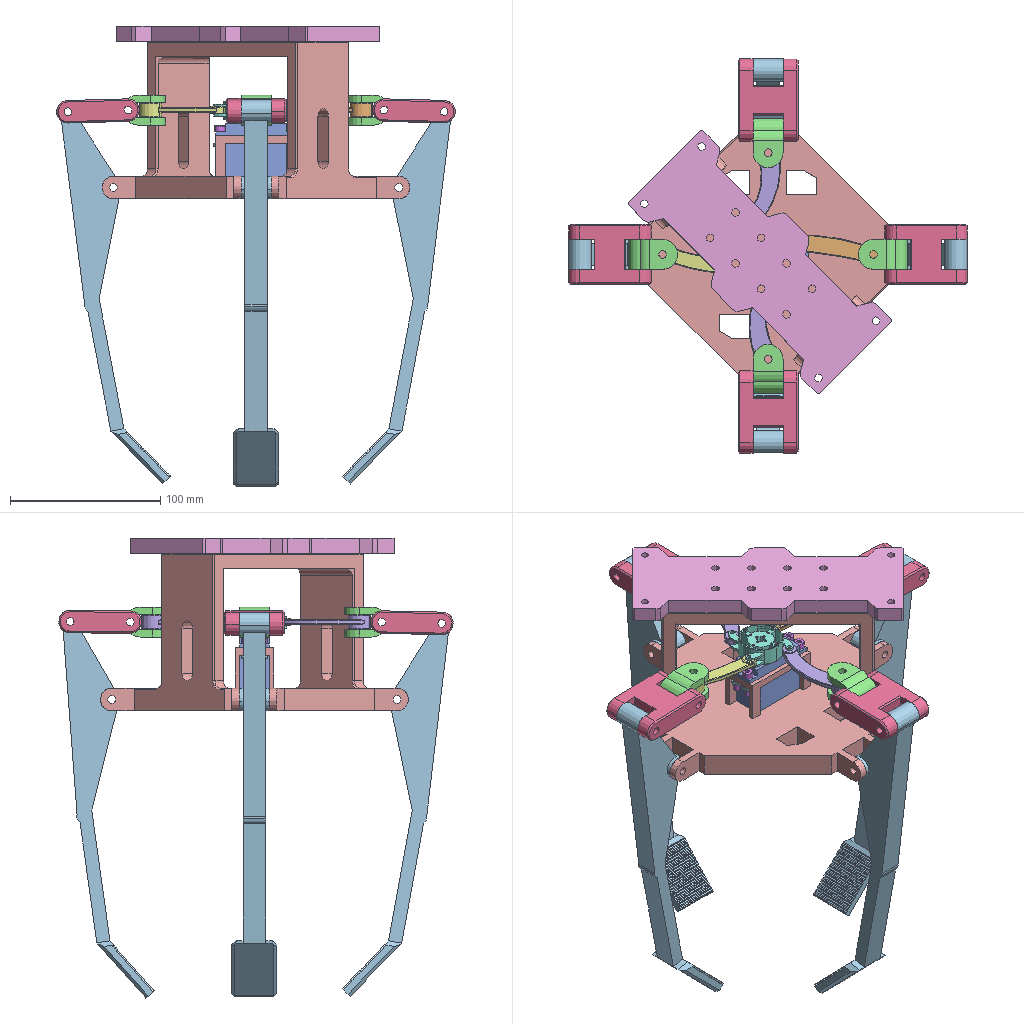Assembly | SolidWorks | 13 different items | 23 placed | box 265 x 262 x 306 mm
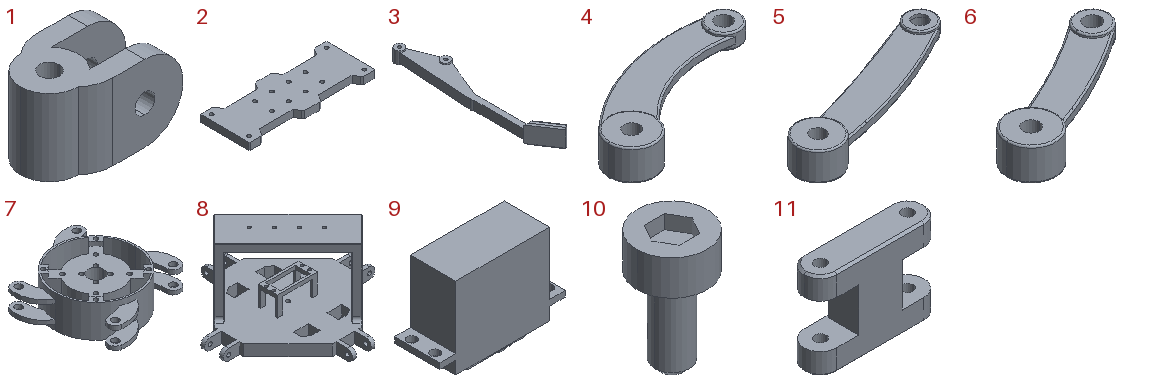Parts list (item | name | quantity | size | volume | features):
1 | - | x4 | 32.5 x 20 x 20 mm | 6873 mm3 | features Fillet 2, ICE 2, Extrusion 1
2 | - | x1 | 180 x 70 x 10 mm | 101775 mm3 | features ICE 3, Chamfer 1, Extrusion 1
3 | - | x4 | 41.169 x 262.682 x 30 mm | 65596 mm3 | features ICE 9, Chamfer 2, Extrusion 1
4 | - | x2 | 60.037 x 31.564 x 10 mm | 3346 mm3 | features Fillet 2, ICE 2, Extrusion 1, MirrorPattern 1
5 | - | x1 | 67.682 x 31.748 x 10 mm | 3550 mm3 | features ICE 2, Extrusion 1, Fillet 1, MirrorPattern 1
6 | - | x1 | 52.377 x 33.585 x 10 mm | 2859 mm3 | features ICE 2, Extrusion 1, Fillet 1, MirrorPattern 1
7 | - | x1 | 40.64 x 40.64 x 12 mm | 4015 mm3 | features ICE 6, CirPattern 1, Extrusion 1, MirrorPattern 1, Scale 1
8 | - | x1 | 205 x 205 x 105 mm | 416769 mm3 | features ICE 14, Fillet 2, MirrorPattern 2, MoveFace 2, Chamfer 1, Extrusion 1, HoleWzd 1
9 | - | x1 | 54 x 19.5 x 43 mm | 29172 mm3 | features MBimport 1
10 | - | x1 | 10 x 10 x 17 mm | 578.21 mm3 | features ICE 2, Chamfer 1, Extrusion 1
11 | - | x4 | 55 x 15 x 40 mm | 20540 mm3 | features ICE 2, Chamfer 1, Extrusion 1
12 | hex thin nut gradeb_iso | x1 | - | - | -
13 | socket head cap screw_iso | x1 | - | - | -
Mates (type | each side: item.copy, entity, surface, feature):
Coincident | 8.1 face plane Boss-Extrude2 | 9.1 face plane Servo(1).STEP<1>
Coincident | 8.1 face plane Boss-Extrude1 | 9.1 face plane Servo(1).STEP<1> | 2 times
Coincident | 8.1 face plane Boss-Extrude7 | 2.1 face plane Boss-Extrude1
Coincident | 8.1 face plane Boss-Extrude6 | 2.1 face plane Cut-Extrude1
Width | 2.1 face plane Boss-Extrude1 | 2.1 face plane Boss-Extrude1 | 8.1 face plane Boss-Extrude3 | 8.1 face plane Boss-Extrude3
Coincident | 9.1 face cylinder Servo(1).STEP<1> | 7.1 edge
Coincident | 9.1 face plane Servo(1).STEP<1> | 7.1 face plane Mirror1
Concentric | 7.1 face cylinder CirPattern1 | 5.1 face cylinder Boss-Extrude2
Coincident | 7.1 face plane Cut-Extrude12 | 5.1 face plane Boss-Extrude3
Concentric | 7.1 face cylinder CirPattern1 | 4.1 face cylinder Boss-Extrude2
Coincident | 7.1 face plane Cut-Extrude12 | 4.1 face plane Boss-Extrude3
Concentric | 7.1 face cylinder Boss-Extrude2 | 4.2 face cylinder Boss-Extrude2
Coincident | 7.1 face plane Cut-Extrude12 | 4.2 face plane Boss-Extrude3
Coincident | 4.2 face plane Boss-Extrude1 | 1.1 face plane Boss-Extrude2
Concentric | 4.2 face cylinder Boss-Extrude1 | 1.1 face cylinder Cut-Extrude1
Coincident | 5.1 face plane Boss-Extrude1 | 1.2 face plane Boss-Extrude2
Concentric | 5.1 face cylinder Boss-Extrude1 | 1.2 face cylinder Cut-Extrude1
Coincident | 4.1 face plane Boss-Extrude1 | 1.3 face plane Boss-Extrude2
Concentric | 4.1 face cylinder Boss-Extrude1 | 1.3 face cylinder Cut-Extrude1
Coincident | 1.4 face plane Boss-Extrude1 | 11.1 face plane Boss-Extrude3
Concentric | 1.4 face cylinder Boss-Extrude1 | 11.1 face cylinder Boss-Extrude3
Coincident | 1.2 face plane Boss-Extrude1 | 11.2 face plane Boss-Extrude3
Concentric | 1.2 face cylinder Boss-Extrude1 | 11.2 face cylinder Boss-Extrude3
Coincident | 1.1 face plane Boss-Extrude1 | 11.3 face plane Boss-Extrude3
Concentric | 1.1 face cylinder Boss-Extrude1 | 11.3 face cylinder Boss-Extrude3
Coincident | 1.3 face plane Boss-Extrude1 | 11.4 face plane Boss-Extrude1
Concentric | 1.3 face cylinder Boss-Extrude1 | 11.4 face cylinder Boss-Extrude1
Coincident | 11.2 face plane Boss-Extrude3 | 3.1 face plane Boss-Extrude1
Concentric | 11.2 face cylinder Boss-Extrude3 | 3.1 face cylinder Cut-Extrude1
Concentric | 8.1 face cylinder Boss-Extrude5 | 3.1 face cylinder Cut-Extrude2
Coincident | 8.1 face plane Mirror2 | 3.1 face plane Boss-Extrude4
Concentric | 11.3 face cylinder Boss-Extrude1 | 3.2 face cylinder Cut-Extrude1
Coincident | 11.3 face plane Boss-Extrude3 | 3.2 face plane Boss-Extrude1
Coincident | 8.1 face plane Mirror1 | 3.2 face plane Boss-Extrude4
Concentric | 8.1 face cylinder Boss-Extrude4 | 3.2 face cylinder Cut-Extrude2
Coincident | 11.4 face plane Boss-Extrude1 | 3.3 face plane Boss-Extrude1
Concentric | 11.4 face cylinder Boss-Extrude1 | 3.3 face cylinder Cut-Extrude1
Coincident | 8.1 face plane Mirror1 | 3.3 face plane Boss-Extrude4
Concentric | 8.1 face cylinder Mirror1 | 3.3 face cylinder Cut-Extrude2
Coincident | 11.1 face plane Boss-Extrude3 | 3.4 face plane Boss-Extrude1
Coincident | 11.1 face plane Boss-Extrude1 | 3.4 face plane Boss-Extrude1
Concentric | 11.1 face cylinder Boss-Extrude1 | 3.4 face cylinder Cut-Extrude1
Concentric | 8.1 face cylinder Mirror2 | 3.4 face cylinder Cut-Extrude2
Coincident | 8.1 face plane Mirror2 | 3.4 face plane Boss-Extrude4
Concentric | 7.1 face cylinder CirPattern1 | 6.1 face cylinder Boss-Extrude2
Coincident | 7.1 face plane Cut-Extrude12 | 6.1 face plane Boss-Extrude3
Coincident | 1.4 face plane Boss-Extrude2 | 6.1 face plane Boss-Extrude1
Concentric | 1.4 face cylinder Cut-Extrude1 | 6.1 face cylinder Boss-Extrude1